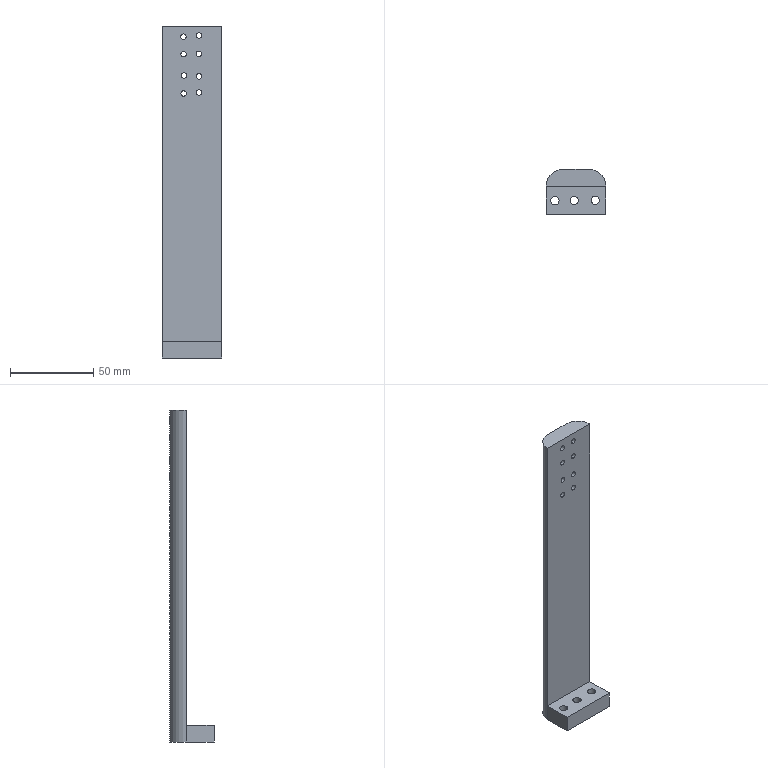Part | STEP file | L3.STEP | 1 solid | 32 faces | box 36 x 26.813 x 200 mm | volume 68195 mm3 | cylinder 24 | plane 8 | commonest cylinder face diameters 3.3 x16 5 x6 20 x2
STEP:
#1=CARTESIAN_POINT('',(-5.181,5.,191.886));
#2=VERTEX_POINT('',#1);
#3=CARTESIAN_POINT('',(-5.181,15.,191.886));
#4=VERTEX_POINT('',#3);
#5=CARTESIAN_POINT('',(-5.181,15.,191.886));
#6=DIRECTION('',(0.,1.,0.));
#7=VECTOR('',#6,1000.);
#8=LINE('',#5,#7);
#9=EDGE_CURVE('',#2,#4,#8,.T.);
#10=ORIENTED_EDGE('',*,*,#9,.F.);
#11=CARTESIAN_POINT('',(-5.181,5.,195.186));
#12=VERTEX_POINT('',#11);
#13=CARTESIAN_POINT('',(-5.181,5.,193.536));
#14=DIRECTION('',(0.,1.,0.));
#15=DIRECTION('',(0.,0.,1.));
#16=AXIS2_PLACEMENT_3D('',#13,#14,#15);
#17=CIRCLE('',#16,1.65);
#18=EDGE_CURVE('',#12,#2,#17,.T.);
#19=ORIENTED_EDGE('',*,*,#18,.F.);
#20=CARTESIAN_POINT('',(-5.181,15.,195.186));
#21=VERTEX_POINT('',#20);
#22=CARTESIAN_POINT('',(-5.181,15.,195.186));
#23=DIRECTION('',(0.,1.,0.));
#24=VECTOR('',#23,1000.);
#25=LINE('',#22,#24);
#26=EDGE_CURVE('',#12,#21,#25,.T.);
#27=ORIENTED_EDGE('',*,*,#26,.T.);
#28=CARTESIAN_POINT('',(-5.181,15.,193.536));
#29=DIRECTION('',(0.,1.,0.));
#30=DIRECTION('',(0.,0.,1.));
#31=AXIS2_PLACEMENT_3D('',#28,#29,#30);
#32=CIRCLE('',#31,1.65);
#33=EDGE_CURVE('',#21,#4,#32,.T.);
#34=ORIENTED_EDGE('',*,*,#33,.T.);
#35=EDGE_LOOP('',(#10,#19,#27,#34));
#36=FACE_OUTER_BOUND('',#35,.T.);
#37=CARTESIAN_POINT('',(-5.181,15.,193.536));
#38=DIRECTION('',(0.,1.,0.));
#39=DIRECTION('',(0.,0.,1.));
#40=AXIS2_PLACEMENT_3D('',#37,#38,#39);
#41=CYLINDRICAL_SURFACE('',#40,1.65);
#42=ADVANCED_FACE('',(#36),#41,.F.);
#43=CARTESIAN_POINT('',(4.086,5.,192.622));
#44=VERTEX_POINT('',#43);
#45=CARTESIAN_POINT('',(4.086,15.,192.622));
#46=VERTEX_POINT('',#45);
#47=CARTESIAN_POINT('',(4.086,15.,192.622));
#48=DIRECTION('',(0.,1.,0.));
#49=VECTOR('',#48,1000.);
#50=LINE('',#47,#49);
#51=EDGE_CURVE('',#44,#46,#50,.T.);
#52=ORIENTED_EDGE('',*,*,#51,.F.);
#53=CARTESIAN_POINT('',(4.086,5.,195.922));
#54=VERTEX_POINT('',#53);
#55=CARTESIAN_POINT('',(4.086,5.,194.272));
#56=DIRECTION('',(0.,1.,0.));
#57=DIRECTION('',(0.,0.,1.));
#58=AXIS2_PLACEMENT_3D('',#55,#56,#57);
#59=CIRCLE('',#58,1.65);
#60=EDGE_CURVE('',#54,#44,#59,.T.);
#61=ORIENTED_EDGE('',*,*,#60,.F.);
#62=CARTESIAN_POINT('',(4.086,15.,195.922));
#63=VERTEX_POINT('',#62);
#64=CARTESIAN_POINT('',(4.086,15.,195.922));
#65=DIRECTION('',(0.,1.,0.));
#66=VECTOR('',#65,1000.);
#67=LINE('',#64,#66);
#68=EDGE_CURVE('',#54,#63,#67,.T.);
#69=ORIENTED_EDGE('',*,*,#68,.T.);
#70=CARTESIAN_POINT('',(4.086,15.,194.272));
#71=DIRECTION('',(0.,1.,0.));
#72=DIRECTION('',(0.,0.,1.));
#73=AXIS2_PLACEMENT_3D('',#70,#71,#72);
#74=CIRCLE('',#73,1.65);
#75=EDGE_CURVE('',#63,#46,#74,.T.);
#76=ORIENTED_EDGE('',*,*,#75,.T.);
#77=EDGE_LOOP('',(#52,#61,#69,#76));
#78=FACE_OUTER_BOUND('',#77,.T.);
#79=CARTESIAN_POINT('',(4.086,15.,194.272));
#80=DIRECTION('',(0.,1.,0.));
#81=DIRECTION('',(0.,0.,1.));
#82=AXIS2_PLACEMENT_3D('',#79,#80,#81);
#83=CYLINDRICAL_SURFACE('',#82,1.65);
#84=ADVANCED_FACE('',(#78),#83,.F.);
#85=CARTESIAN_POINT('',(-5.004,5.,181.372));
#86=VERTEX_POINT('',#85);
#87=CARTESIAN_POINT('',(-5.004,15.,181.372));
#88=VERTEX_POINT('',#87);
#89=CARTESIAN_POINT('',(-5.004,15.,181.372));
#90=DIRECTION('',(0.,1.,0.));
#91=VECTOR('',#90,1000.);
#92=LINE('',#89,#91);
#93=EDGE_CURVE('',#86,#88,#92,.T.);
#94=ORIENTED_EDGE('',*,*,#93,.F.);
#95=CARTESIAN_POINT('',(-5.004,5.,184.672));
#96=VERTEX_POINT('',#95);
#97=CARTESIAN_POINT('',(-5.004,5.,183.022));
#98=DIRECTION('',(0.,1.,0.));
#99=DIRECTION('',(0.,0.,1.));
#100=AXIS2_PLACEMENT_3D('',#97,#98,#99);
#101=CIRCLE('',#100,1.65);
#102=EDGE_CURVE('',#96,#86,#101,.T.);
#103=ORIENTED_EDGE('',*,*,#102,.F.);
#104=CARTESIAN_POINT('',(-5.004,15.,184.672));
#105=VERTEX_POINT('',#104);
#106=CARTESIAN_POINT('',(-5.004,15.,184.672));
#107=DIRECTION('',(0.,1.,0.));
#108=VECTOR('',#107,1000.);
#109=LINE('',#106,#108);
#110=EDGE_CURVE('',#96,#105,#109,.T.);
#111=ORIENTED_EDGE('',*,*,#110,.T.);
#112=CARTESIAN_POINT('',(-5.004,15.,183.022));
#113=DIRECTION('',(0.,1.,0.));
#114=DIRECTION('',(0.,0.,1.));
#115=AXIS2_PLACEMENT_3D('',#112,#113,#114);
#116=CIRCLE('',#115,1.65);
#117=EDGE_CURVE('',#105,#88,#116,.T.);
#118=ORIENTED_EDGE('',*,*,#117,.T.);
#119=EDGE_LOOP('',(#94,#103,#111,#118));
#120=FACE_OUTER_BOUND('',#119,.T.);
#121=CARTESIAN_POINT('',(-5.004,15.,183.022));
#122=DIRECTION('',(0.,1.,0.));
#123=DIRECTION('',(0.,0.,1.));
#124=AXIS2_PLACEMENT_3D('',#121,#122,#123);
#125=CYLINDRICAL_SURFACE('',#124,1.65);
#126=ADVANCED_FACE('',(#120),#125,.F.);
#127=CARTESIAN_POINT('',(4.079,5.,181.598));
#128=VERTEX_POINT('',#127);
#129=CARTESIAN_POINT('',(4.079,15.,181.598));
#130=VERTEX_POINT('',#129);
#131=CARTESIAN_POINT('',(4.079,15.,181.598));
#132=DIRECTION('',(0.,1.,0.));
#133=VECTOR('',#132,1000.);
#134=LINE('',#131,#133);
#135=EDGE_CURVE('',#128,#130,#134,.T.);
#136=ORIENTED_EDGE('',*,*,#135,.F.);
#137=CARTESIAN_POINT('',(4.079,5.,184.898));
#138=VERTEX_POINT('',#137);
#139=CARTESIAN_POINT('',(4.079,5.,183.248));
#140=DIRECTION('',(0.,1.,0.));
#141=DIRECTION('',(0.,0.,1.));
#142=AXIS2_PLACEMENT_3D('',#139,#140,#141);
#143=CIRCLE('',#142,1.65);
#144=EDGE_CURVE('',#138,#128,#143,.T.);
#145=ORIENTED_EDGE('',*,*,#144,.F.);
#146=CARTESIAN_POINT('',(4.079,15.,184.898));
#147=VERTEX_POINT('',#146);
#148=CARTESIAN_POINT('',(4.079,15.,184.898));
#149=DIRECTION('',(0.,1.,0.));
#150=VECTOR('',#149,1000.);
#151=LINE('',#148,#150);
#152=EDGE_CURVE('',#138,#147,#151,.T.);
#153=ORIENTED_EDGE('',*,*,#152,.T.);
#154=CARTESIAN_POINT('',(4.079,15.,183.248));
#155=DIRECTION('',(0.,1.,0.));
#156=DIRECTION('',(0.,0.,1.));
#157=AXIS2_PLACEMENT_3D('',#154,#155,#156);
#158=CIRCLE('',#157,1.65);
#159=EDGE_CURVE('',#147,#130,#158,.T.);
#160=ORIENTED_EDGE('',*,*,#159,.T.);
#161=EDGE_LOOP('',(#136,#145,#153,#160));
#162=FACE_OUTER_BOUND('',#161,.T.);
#163=CARTESIAN_POINT('',(4.079,15.,183.248));
#164=DIRECTION('',(0.,1.,0.));
#165=DIRECTION('',(0.,0.,1.));
#166=AXIS2_PLACEMENT_3D('',#163,#164,#165);
#167=CYLINDRICAL_SURFACE('',#166,1.65);
#168=ADVANCED_FACE('',(#162),#167,.F.);
#169=CARTESIAN_POINT('',(4.196,5.,168.));
#170=VERTEX_POINT('',#169);
#171=CARTESIAN_POINT('',(4.196,15.,168.));
#172=VERTEX_POINT('',#171);
#173=CARTESIAN_POINT('',(4.196,15.,168.));
#174=DIRECTION('',(0.,1.,0.));
#175=VECTOR('',#174,1000.);
#176=LINE('',#173,#175);
#177=EDGE_CURVE('',#170,#172,#176,.T.);
#178=ORIENTED_EDGE('',*,*,#177,.F.);
#179=CARTESIAN_POINT('',(4.196,5.,171.3));
#180=VERTEX_POINT('',#179);
#181=CARTESIAN_POINT('',(4.196,5.,169.65));
#182=DIRECTION('',(0.,1.,0.));
#183=DIRECTION('',(0.,0.,1.));
#184=AXIS2_PLACEMENT_3D('',#181,#182,#183);
#185=CIRCLE('',#184,1.65);
#186=EDGE_CURVE('',#180,#170,#185,.T.);
#187=ORIENTED_EDGE('',*,*,#186,.F.);
#188=CARTESIAN_POINT('',(4.196,15.,171.3));
#189=VERTEX_POINT('',#188);
#190=CARTESIAN_POINT('',(4.196,15.,171.3));
#191=DIRECTION('',(0.,1.,0.));
#192=VECTOR('',#191,1000.);
#193=LINE('',#190,#192);
#194=EDGE_CURVE('',#180,#189,#193,.T.);
#195=ORIENTED_EDGE('',*,*,#194,.T.);
#196=CARTESIAN_POINT('',(4.196,15.,169.65));
#197=DIRECTION('',(0.,1.,0.));
#198=DIRECTION('',(0.,0.,1.));
#199=AXIS2_PLACEMENT_3D('',#196,#197,#198);
#200=CIRCLE('',#199,1.65);
#201=EDGE_CURVE('',#189,#172,#200,.T.);
#202=ORIENTED_EDGE('',*,*,#201,.T.);
#203=EDGE_LOOP('',(#178,#187,#195,#202));
#204=FACE_OUTER_BOUND('',#203,.T.);
#205=CARTESIAN_POINT('',(4.196,15.,169.65));
#206=DIRECTION('',(0.,1.,0.));
#207=DIRECTION('',(0.,0.,1.));
#208=AXIS2_PLACEMENT_3D('',#205,#206,#207);
#209=CYLINDRICAL_SURFACE('',#208,1.65);
#210=ADVANCED_FACE('',(#204),#209,.F.);
#211=CARTESIAN_POINT('',(-4.737,5.,168.514));
#212=VERTEX_POINT('',#211);
#213=CARTESIAN_POINT('',(-4.737,15.,168.514));
#214=VERTEX_POINT('',#213);
#215=CARTESIAN_POINT('',(-4.737,15.,168.514));
#216=DIRECTION('',(0.,1.,0.));
#217=VECTOR('',#216,1000.);
#218=LINE('',#215,#217);
#219=EDGE_CURVE('',#212,#214,#218,.T.);
#220=ORIENTED_EDGE('',*,*,#219,.F.);
#221=CARTESIAN_POINT('',(-4.737,5.,171.814));
#222=VERTEX_POINT('',#221);
#223=CARTESIAN_POINT('',(-4.737,5.,170.164));
#224=DIRECTION('',(0.,1.,0.));
#225=DIRECTION('',(0.,0.,1.));
#226=AXIS2_PLACEMENT_3D('',#223,#224,#225);
#227=CIRCLE('',#226,1.65);
#228=EDGE_CURVE('',#222,#212,#227,.T.);
#229=ORIENTED_EDGE('',*,*,#228,.F.);
#230=CARTESIAN_POINT('',(-4.737,15.,171.814));
#231=VERTEX_POINT('',#230);
#232=CARTESIAN_POINT('',(-4.737,15.,171.814));
#233=DIRECTION('',(0.,1.,0.));
#234=VECTOR('',#233,1000.);
#235=LINE('',#232,#234);
#236=EDGE_CURVE('',#222,#231,#235,.T.);
#237=ORIENTED_EDGE('',*,*,#236,.T.);
#238=CARTESIAN_POINT('',(-4.737,15.,170.164));
#239=DIRECTION('',(0.,1.,0.));
#240=DIRECTION('',(0.,0.,1.));
#241=AXIS2_PLACEMENT_3D('',#238,#239,#240);
#242=CIRCLE('',#241,1.65);
#243=EDGE_CURVE('',#231,#214,#242,.T.);
#244=ORIENTED_EDGE('',*,*,#243,.T.);
#245=EDGE_LOOP('',(#220,#229,#237,#244));
#246=FACE_OUTER_BOUND('',#245,.T.);
#247=CARTESIAN_POINT('',(-4.737,15.,170.164));
#248=DIRECTION('',(0.,1.,0.));
#249=DIRECTION('',(0.,0.,1.));
#250=AXIS2_PLACEMENT_3D('',#247,#248,#249);
#251=CYLINDRICAL_SURFACE('',#250,1.65);
#252=ADVANCED_FACE('',(#246),#251,.F.);
#253=CARTESIAN_POINT('',(4.08,5.,158.292));
#254=VERTEX_POINT('',#253);
#255=CARTESIAN_POINT('',(4.08,15.,158.292));
#256=VERTEX_POINT('',#255);
#257=CARTESIAN_POINT('',(4.08,15.,158.292));
#258=DIRECTION('',(0.,1.,0.));
#259=VECTOR('',#258,1000.);
#260=LINE('',#257,#259);
#261=EDGE_CURVE('',#254,#256,#260,.T.);
#262=ORIENTED_EDGE('',*,*,#261,.F.);
#263=CARTESIAN_POINT('',(4.08,5.,161.592));
#264=VERTEX_POINT('',#263);
#265=CARTESIAN_POINT('',(4.08,5.,159.942));
#266=DIRECTION('',(0.,1.,0.));
#267=DIRECTION('',(0.,0.,1.));
#268=AXIS2_PLACEMENT_3D('',#265,#266,#267);
#269=CIRCLE('',#268,1.65);
#270=EDGE_CURVE('',#264,#254,#269,.T.);
#271=ORIENTED_EDGE('',*,*,#270,.F.);
#272=CARTESIAN_POINT('',(4.08,15.,161.592));
#273=VERTEX_POINT('',#272);
#274=CARTESIAN_POINT('',(4.08,15.,161.592));
#275=DIRECTION('',(0.,1.,0.));
#276=VECTOR('',#275,1000.);
#277=LINE('',#274,#276);
#278=EDGE_CURVE('',#264,#273,#277,.T.);
#279=ORIENTED_EDGE('',*,*,#278,.T.);
#280=CARTESIAN_POINT('',(4.08,15.,159.942));
#281=DIRECTION('',(0.,1.,0.));
#282=DIRECTION('',(0.,0.,1.));
#283=AXIS2_PLACEMENT_3D('',#280,#281,#282);
#284=CIRCLE('',#283,1.65);
#285=EDGE_CURVE('',#273,#256,#284,.T.);
#286=ORIENTED_EDGE('',*,*,#285,.T.);
#287=EDGE_LOOP('',(#262,#271,#279,#286));
#288=FACE_OUTER_BOUND('',#287,.T.);
#289=CARTESIAN_POINT('',(4.08,15.,159.942));
#290=DIRECTION('',(0.,1.,0.));
#291=DIRECTION('',(0.,0.,1.));
#292=AXIS2_PLACEMENT_3D('',#289,#290,#291);
#293=CYLINDRICAL_SURFACE('',#292,1.65);
#294=ADVANCED_FACE('',(#288),#293,.F.);
#295=CARTESIAN_POINT('',(-5.03,5.,157.667));
#296=VERTEX_POINT('',#295);
#297=CARTESIAN_POINT('',(-5.03,15.,157.667));
#298=VERTEX_POINT('',#297);
#299=CARTESIAN_POINT('',(-5.03,15.,157.667));
#300=DIRECTION('',(0.,1.,0.));
#301=VECTOR('',#300,1000.);
#302=LINE('',#299,#301);
#303=EDGE_CURVE('',#296,#298,#302,.T.);
#304=ORIENTED_EDGE('',*,*,#303,.F.);
#305=CARTESIAN_POINT('',(-5.03,5.,160.967));
#306=VERTEX_POINT('',#305);
#307=CARTESIAN_POINT('',(-5.03,5.,159.317));
#308=DIRECTION('',(0.,1.,0.));
#309=DIRECTION('',(0.,0.,1.));
#310=AXIS2_PLACEMENT_3D('',#307,#308,#309);
#311=CIRCLE('',#310,1.65);
#312=EDGE_CURVE('',#306,#296,#311,.T.);
#313=ORIENTED_EDGE('',*,*,#312,.F.);
#314=CARTESIAN_POINT('',(-5.03,15.,160.967));
#315=VERTEX_POINT('',#314);
#316=CARTESIAN_POINT('',(-5.03,15.,160.967));
#317=DIRECTION('',(0.,1.,0.));
#318=VECTOR('',#317,1000.);
#319=LINE('',#316,#318);
#320=EDGE_CURVE('',#306,#315,#319,.T.);
#321=ORIENTED_EDGE('',*,*,#320,.T.);
#322=CARTESIAN_POINT('',(-5.03,15.,159.317));
#323=DIRECTION('',(0.,1.,0.));
#324=DIRECTION('',(0.,0.,1.));
#325=AXIS2_PLACEMENT_3D('',#322,#323,#324);
#326=CIRCLE('',#325,1.65);
#327=EDGE_CURVE('',#315,#298,#326,.T.);
#328=ORIENTED_EDGE('',*,*,#327,.T.);
#329=EDGE_LOOP('',(#304,#313,#321,#328));
#330=FACE_OUTER_BOUND('',#329,.T.);
#331=CARTESIAN_POINT('',(-5.03,15.,159.317));
#332=DIRECTION('',(0.,1.,0.));
#333=DIRECTION('',(0.,0.,1.));
#334=AXIS2_PLACEMENT_3D('',#331,#332,#333);
#335=CYLINDRICAL_SURFACE('',#334,1.65);
#336=ADVANCED_FACE('',(#330),#335,.F.);
#337=CARTESIAN_POINT('',(14.125,-3.204,10.));
#338=VERTEX_POINT('',#337);
#339=CARTESIAN_POINT('',(14.125,-3.204,0.));
#340=VERTEX_POINT('',#339);
#341=CARTESIAN_POINT('',(14.125,-3.204,0.));
#342=DIRECTION('',(0.,0.,-1.));
#343=VECTOR('',#342,1000.);
#344=LINE('',#341,#343);
#345=EDGE_CURVE('',#338,#340,#344,.T.);
#346=ORIENTED_EDGE('',*,*,#345,.F.);
#347=CARTESIAN_POINT('',(9.125,-3.204,10.));
#348=VERTEX_POINT('',#347);
#349=CARTESIAN_POINT('',(11.625,-3.204,10.));
#350=DIRECTION('',(0.,0.,-1.));
#351=DIRECTION('',(-1.,0.,0.));
#352=AXIS2_PLACEMENT_3D('',#349,#350,#351);
#353=CIRCLE('',#352,2.5);
#354=EDGE_CURVE('',#348,#338,#353,.T.);
#355=ORIENTED_EDGE('',*,*,#354,.F.);
#356=CARTESIAN_POINT('',(9.125,-3.204,0.));
#357=VERTEX_POINT('',#356);
#358=CARTESIAN_POINT('',(9.125,-3.204,0.));
#359=DIRECTION('',(0.,0.,-1.));
#360=VECTOR('',#359,1000.);
#361=LINE('',#358,#360);
#362=EDGE_CURVE('',#348,#357,#361,.T.);
#363=ORIENTED_EDGE('',*,*,#362,.T.);
#364=CARTESIAN_POINT('',(11.625,-3.204,0.));
#365=DIRECTION('',(0.,0.,-1.));
#366=DIRECTION('',(-1.,0.,0.));
#367=AXIS2_PLACEMENT_3D('',#364,#365,#366);
#368=CIRCLE('',#367,2.5);
#369=EDGE_CURVE('',#357,#340,#368,.T.);
#370=ORIENTED_EDGE('',*,*,#369,.T.);
#371=EDGE_LOOP('',(#346,#355,#363,#370));
#372=FACE_OUTER_BOUND('',#371,.T.);
#373=CARTESIAN_POINT('',(11.625,-3.204,0.));
#374=DIRECTION('',(0.,0.,-1.));
#375=DIRECTION('',(-1.,0.,0.));
#376=AXIS2_PLACEMENT_3D('',#373,#374,#375);
#377=CYLINDRICAL_SURFACE('',#376,2.5);
#378=ADVANCED_FACE('',(#372),#377,.F.);
#379=CARTESIAN_POINT('',(1.426,-3.367,10.));
#380=VERTEX_POINT('',#379);
#381=CARTESIAN_POINT('',(1.426,-3.367,0.));
#382=VERTEX_POINT('',#381);
#383=CARTESIAN_POINT('',(1.426,-3.367,0.));
#384=DIRECTION('',(0.,0.,-1.));
#385=VECTOR('',#384,1000.);
#386=LINE('',#383,#385);
#387=EDGE_CURVE('',#380,#382,#386,.T.);
#388=ORIENTED_EDGE('',*,*,#387,.F.);
#389=CARTESIAN_POINT('',(-3.574,-3.367,10.));
#390=VERTEX_POINT('',#389);
#391=CARTESIAN_POINT('',(-1.074,-3.367,10.));
#392=DIRECTION('',(0.,0.,-1.));
#393=DIRECTION('',(-1.,0.,0.));
#394=AXIS2_PLACEMENT_3D('',#391,#392,#393);
#395=CIRCLE('',#394,2.5);
#396=EDGE_CURVE('',#390,#380,#395,.T.);
#397=ORIENTED_EDGE('',*,*,#396,.F.);
#398=CARTESIAN_POINT('',(-3.574,-3.367,0.));
#399=VERTEX_POINT('',#398);
#400=CARTESIAN_POINT('',(-3.574,-3.367,0.));
#401=DIRECTION('',(0.,0.,-1.));
#402=VECTOR('',#401,1000.);
#403=LINE('',#400,#402);
#404=EDGE_CURVE('',#390,#399,#403,.T.);
#405=ORIENTED_EDGE('',*,*,#404,.T.);
#406=CARTESIAN_POINT('',(-1.074,-3.367,0.));
#407=DIRECTION('',(0.,0.,-1.));
#408=DIRECTION('',(-1.,0.,0.));
#409=AXIS2_PLACEMENT_3D('',#406,#407,#408);
#410=CIRCLE('',#409,2.5);
#411=EDGE_CURVE('',#399,#382,#410,.T.);
#412=ORIENTED_EDGE('',*,*,#411,.T.);
#413=EDGE_LOOP('',(#388,#397,#405,#412));
#414=FACE_OUTER_BOUND('',#413,.T.);
#415=CARTESIAN_POINT('',(-1.074,-3.367,0.));
#416=DIRECTION('',(0.,0.,-1.));
#417=DIRECTION('',(-1.,0.,0.));
#418=AXIS2_PLACEMENT_3D('',#415,#416,#417);
#419=CYLINDRICAL_SURFACE('',#418,2.5);
#420=ADVANCED_FACE('',(#414),#419,.F.);
#421=CARTESIAN_POINT('',(-10.172,-3.581,10.));
#422=VERTEX_POINT('',#421);
#423=CARTESIAN_POINT('',(-10.172,-3.581,0.));
#424=VERTEX_POINT('',#423);
#425=CARTESIAN_POINT('',(-10.172,-3.581,0.));
#426=DIRECTION('',(0.,0.,-1.));
#427=VECTOR('',#426,1000.);
#428=LINE('',#425,#427);
#429=EDGE_CURVE('',#422,#424,#428,.T.);
#430=ORIENTED_EDGE('',*,*,#429,.F.);
#431=CARTESIAN_POINT('',(-15.172,-3.581,10.));
#432=VERTEX_POINT('',#431);
#433=CARTESIAN_POINT('',(-12.672,-3.581,10.));
#434=DIRECTION('',(0.,0.,-1.));
#435=DIRECTION('',(-1.,0.,0.));
#436=AXIS2_PLACEMENT_3D('',#433,#434,#435);
#437=CIRCLE('',#436,2.5);
#438=EDGE_CURVE('',#432,#422,#437,.T.);
#439=ORIENTED_EDGE('',*,*,#438,.F.);
#440=CARTESIAN_POINT('',(-15.172,-3.581,0.));
#441=VERTEX_POINT('',#440);
#442=CARTESIAN_POINT('',(-15.172,-3.581,0.));
#443=DIRECTION('',(0.,0.,-1.));
#444=VECTOR('',#443,1000.);
#445=LINE('',#442,#444);
#446=EDGE_CURVE('',#432,#441,#445,.T.);
#447=ORIENTED_EDGE('',*,*,#446,.T.);
#448=CARTESIAN_POINT('',(-12.672,-3.581,0.));
#449=DIRECTION('',(0.,0.,-1.));
#450=DIRECTION('',(-1.,0.,0.));
#451=AXIS2_PLACEMENT_3D('',#448,#449,#450);
#452=CIRCLE('',#451,2.5);
#453=EDGE_CURVE('',#441,#424,#452,.T.);
#454=ORIENTED_EDGE('',*,*,#453,.T.);
#455=EDGE_LOOP('',(#430,#439,#447,#454));
#456=FACE_OUTER_BOUND('',#455,.T.);
#457=CARTESIAN_POINT('',(-12.672,-3.581,0.));
#458=DIRECTION('',(0.,0.,-1.));
#459=DIRECTION('',(-1.,0.,0.));
#460=AXIS2_PLACEMENT_3D('',#457,#458,#459);
#461=CYLINDRICAL_SURFACE('',#460,2.5);
#462=ADVANCED_FACE('',(#456),#461,.F.);
#463=ORIENTED_EDGE('',*,*,#438,.T.);
#464=CARTESIAN_POINT('',(-12.672,-3.581,10.));
#465=DIRECTION('',(0.,0.,-1.));
#466=DIRECTION('',(-1.,0.,0.));
#467=AXIS2_PLACEMENT_3D('',#464,#465,#466);
#468=CIRCLE('',#467,2.5);
#469=EDGE_CURVE('',#422,#432,#468,.T.);
#470=ORIENTED_EDGE('',*,*,#469,.T.);
#471=EDGE_LOOP('',(#463,#470));
#472=FACE_BOUND('',#471,.T.);
#473=ORIENTED_EDGE('',*,*,#396,.T.);
#474=CARTESIAN_POINT('',(-1.074,-3.367,10.));
#475=DIRECTION('',(0.,0.,-1.));
#476=DIRECTION('',(-1.,0.,0.));
#477=AXIS2_PLACEMENT_3D('',#474,#475,#476);
#478=CIRCLE('',#477,2.5);
#479=EDGE_CURVE('',#380,#390,#478,.T.);
#480=ORIENTED_EDGE('',*,*,#479,.T.);
#481=EDGE_LOOP('',(#473,#480));
#482=FACE_BOUND('',#481,.T.);
#483=ORIENTED_EDGE('',*,*,#354,.T.);
#484=CARTESIAN_POINT('',(11.625,-3.204,10.));
#485=DIRECTION('',(0.,0.,-1.));
#486=DIRECTION('',(-1.,0.,0.));
#487=AXIS2_PLACEMENT_3D('',#484,#485,#486);
#488=CIRCLE('',#487,2.5);
#489=EDGE_CURVE('',#338,#348,#488,.T.);
#490=ORIENTED_EDGE('',*,*,#489,.T.);
#491=EDGE_LOOP('',(#483,#490));
#492=FACE_BOUND('',#491,.T.);
#493=CARTESIAN_POINT('',(18.,5.,10.));
#494=VERTEX_POINT('',#493);
#495=CARTESIAN_POINT('',(18.,-11.813,10.));
#496=VERTEX_POINT('',#495);
#497=CARTESIAN_POINT('',(18.,5.,10.));
#498=DIRECTION('',(0.,-1.,0.));
#499=VECTOR('',#498,1000.);
#500=LINE('',#497,#499);
#501=EDGE_CURVE('',#494,#496,#500,.T.);
#502=ORIENTED_EDGE('',*,*,#501,.F.);
#503=CARTESIAN_POINT('',(-18.,5.,10.));
#504=VERTEX_POINT('',#503);
#505=CARTESIAN_POINT('',(18.,5.,10.));
#506=DIRECTION('',(1.,0.,0.));
#507=VECTOR('',#506,1000.);
#508=LINE('',#505,#507);
#509=EDGE_CURVE('',#504,#494,#508,.T.);
#510=ORIENTED_EDGE('',*,*,#509,.F.);
#511=CARTESIAN_POINT('',(-18.,-11.813,10.));
#512=VERTEX_POINT('',#511);
#513=CARTESIAN_POINT('',(-18.,5.,10.));
#514=DIRECTION('',(0.,1.,0.));
#515=VECTOR('',#514,1000.);
#516=LINE('',#513,#515);
#517=EDGE_CURVE('',#512,#504,#516,.T.);
#518=ORIENTED_EDGE('',*,*,#517,.F.);
#519=CARTESIAN_POINT('',(18.,-11.813,10.));
#520=DIRECTION('',(-1.,0.,0.));
#521=VECTOR('',#520,1000.);
#522=LINE('',#519,#521);
#523=EDGE_CURVE('',#496,#512,#522,.T.);
#524=ORIENTED_EDGE('',*,*,#523,.F.);
#525=EDGE_LOOP('',(#502,#510,#518,#524));
#526=FACE_OUTER_BOUND('',#525,.T.);
#527=CARTESIAN_POINT('',(0.,0.,10.));
#528=DIRECTION('',(0.,0.,-1.));
#529=DIRECTION('',(0.,-1.,0.));
#530=AXIS2_PLACEMENT_3D('',#527,#528,#529);
#531=PLANE('',#530);
#532=ADVANCED_FACE('',(#472,#482,#492,#526),#531,.F.);
#533=CARTESIAN_POINT('',(18.,-11.813,0.));
#534=VERTEX_POINT('',#533);
#535=CARTESIAN_POINT('',(-18.,-11.813,0.));
#536=VERTEX_POINT('',#535);
#537=CARTESIAN_POINT('',(18.,-11.813,0.));
#538=DIRECTION('',(-1.,0.,0.));
#539=VECTOR('',#538,1000.);
#540=LINE('',#537,#539);
#541=EDGE_CURVE('',#534,#536,#540,.T.);
#542=ORIENTED_EDGE('',*,*,#541,.F.);
#543=CARTESIAN_POINT('',(18.,-11.813,10.));
#544=DIRECTION('',(0.,0.,-1.));
#545=VECTOR('',#544,1000.);
#546=LINE('',#543,#545);
#547=EDGE_CURVE('',#496,#534,#546,.T.);
#548=ORIENTED_EDGE('',*,*,#547,.F.);
#549=ORIENTED_EDGE('',*,*,#523,.T.);
#550=CARTESIAN_POINT('',(-18.,-11.813,10.));
#551=DIRECTION('',(0.,0.,-1.));
#552=VECTOR('',#551,1000.);
#553=LINE('',#550,#552);
#554=EDGE_CURVE('',#512,#536,#553,.T.);
#555=ORIENTED_EDGE('',*,*,#554,.T.);
#556=EDGE_LOOP('',(#542,#548,#549,#555));
#557=FACE_OUTER_BOUND('',#556,.T.);
#558=CARTESIAN_POINT('',(18.,-11.813,10.));
#559=DIRECTION('',(0.,-1.,0.));
#560=DIRECTION('',(0.,0.,-1.));
#561=AXIS2_PLACEMENT_3D('',#558,#559,#560);
#562=PLANE('',#561);
#563=ADVANCED_FACE('',(#557),#562,.T.);
#564=CARTESIAN_POINT('',(-18.,5.,0.));
#565=VERTEX_POINT('',#564);
#566=CARTESIAN_POINT('',(-18.,5.,0.));
#567=DIRECTION('',(0.,1.,0.));
#568=VECTOR('',#567,1000.);
#569=LINE('',#566,#568);
#570=EDGE_CURVE('',#536,#565,#569,.T.);
#571=ORIENTED_EDGE('',*,*,#570,.F.);
#572=ORIENTED_EDGE('',*,*,#554,.F.);
#573=ORIENTED_EDGE('',*,*,#517,.T.);
#574=CARTESIAN_POINT('',(-18.,5.,10.));
#575=DIRECTION('',(0.,0.,-1.));
#576=VECTOR('',#575,1000.);
#577=LINE('',#574,#576);
#578=EDGE_CURVE('',#504,#565,#577,.T.);
#579=ORIENTED_EDGE('',*,*,#578,.T.);
#580=EDGE_LOOP('',(#571,#572,#573,#579));
#581=FACE_OUTER_BOUND('',#580,.T.);
#582=CARTESIAN_POINT('',(-18.,5.,10.));
#583=DIRECTION('',(-1.,0.,0.));
#584=DIRECTION('',(0.,0.,1.));
#585=AXIS2_PLACEMENT_3D('',#582,#583,#584);
#586=PLANE('',#585);
#587=ADVANCED_FACE('',(#581),#586,.T.);
#588=CARTESIAN_POINT('',(18.,5.,0.));
#589=VERTEX_POINT('',#588);
#590=CARTESIAN_POINT('',(18.,5.,0.));
#591=DIRECTION('',(0.,-1.,0.));
#592=VECTOR('',#591,1000.);
#593=LINE('',#590,#592);
#594=EDGE_CURVE('',#589,#534,#593,.T.);
#595=ORIENTED_EDGE('',*,*,#594,.F.);
#596=CARTESIAN_POINT('',(18.,5.,10.));
#597=DIRECTION('',(0.,0.,-1.));
#598=VECTOR('',#597,1000.);
#599=LINE('',#596,#598);
#600=EDGE_CURVE('',#494,#589,#599,.T.);
#601=ORIENTED_EDGE('',*,*,#600,.F.);
#602=ORIENTED_EDGE('',*,*,#501,.T.);
#603=ORIENTED_EDGE('',*,*,#547,.T.);
#604=EDGE_LOOP('',(#595,#601,#602,#603));
#605=FACE_OUTER_BOUND('',#604,.T.);
#606=CARTESIAN_POINT('',(18.,5.,10.));
#607=DIRECTION('',(1.,0.,0.));
#608=DIRECTION('',(0.,1.,0.));
#609=AXIS2_PLACEMENT_3D('',#606,#607,#608);
#610=PLANE('',#609);
#611=ADVANCED_FACE('',(#605),#610,.T.);
#612=ORIENTED_EDGE('',*,*,#453,.F.);
#613=CARTESIAN_POINT('',(-12.672,-3.581,0.));
#614=DIRECTION('',(0.,0.,-1.));
#615=DIRECTION('',(-1.,0.,0.));
#616=AXIS2_PLACEMENT_3D('',#613,#614,#615);
#617=CIRCLE('',#616,2.5);
#618=EDGE_CURVE('',#424,#441,#617,.T.);
#619=ORIENTED_EDGE('',*,*,#618,.F.);
#620=EDGE_LOOP('',(#612,#619));
#621=FACE_BOUND('',#620,.T.);
#622=ORIENTED_EDGE('',*,*,#411,.F.);
#623=CARTESIAN_POINT('',(-1.074,-3.367,0.));
#624=DIRECTION('',(0.,0.,-1.));
#625=DIRECTION('',(-1.,0.,0.));
#626=AXIS2_PLACEMENT_3D('',#623,#624,#625);
#627=CIRCLE('',#626,2.5);
#628=EDGE_CURVE('',#382,#399,#627,.T.);
#629=ORIENTED_EDGE('',*,*,#628,.F.);
#630=EDGE_LOOP('',(#622,#629));
#631=FACE_BOUND('',#630,.T.);
#632=ORIENTED_EDGE('',*,*,#369,.F.);
#633=CARTESIAN_POINT('',(11.625,-3.204,0.));
#634=DIRECTION('',(0.,0.,-1.));
#635=DIRECTION('',(-1.,0.,0.));
#636=AXIS2_PLACEMENT_3D('',#633,#634,#635);
#637=CIRCLE('',#636,2.5);
#638=EDGE_CURVE('',#340,#357,#637,.T.);
#639=ORIENTED_EDGE('',*,*,#638,.F.);
#640=EDGE_LOOP('',(#632,#639));
#641=FACE_BOUND('',#640,.T.);
#642=CARTESIAN_POINT('',(-8.,15.,0.));
#643=VERTEX_POINT('',#642);
#644=CARTESIAN_POINT('',(8.,15.,0.));
#645=VERTEX_POINT('',#644);
#646=CARTESIAN_POINT('',(0.,15.,0.));
#647=DIRECTION('',(1.,0.,0.));
#648=VECTOR('',#647,1000.);
#649=LINE('',#646,#648);
#650=EDGE_CURVE('',#643,#645,#649,.T.);
#651=ORIENTED_EDGE('',*,*,#650,.T.);
#652=CARTESIAN_POINT('',(8.,5.,0.));
#653=DIRECTION('',(0.,0.,-1.));
#654=DIRECTION('',(1.,0.,0.));
#655=AXIS2_PLACEMENT_3D('',#652,#653,#654);
#656=CIRCLE('',#655,10.);
#657=EDGE_CURVE('',#645,#589,#656,.T.);
#658=ORIENTED_EDGE('',*,*,#657,.T.);
#659=ORIENTED_EDGE('',*,*,#594,.T.);
#660=ORIENTED_EDGE('',*,*,#541,.T.);
#661=ORIENTED_EDGE('',*,*,#570,.T.);
#662=CARTESIAN_POINT('',(-8.,5.,0.));
#663=DIRECTION('',(0.,0.,1.));
#664=DIRECTION('',(1.,0.,0.));
#665=AXIS2_PLACEMENT_3D('',#662,#663,#664);
#666=CIRCLE('',#665,10.);
#667=EDGE_CURVE('',#643,#565,#666,.T.);
#668=ORIENTED_EDGE('',*,*,#667,.F.);
#669=EDGE_LOOP('',(#651,#658,#659,#660,#661,#668));
#670=FACE_OUTER_BOUND('',#669,.T.);
#671=CARTESIAN_POINT('',(0.,0.,0.));
#672=DIRECTION('',(0.,0.,1.));
#673=DIRECTION('',(1.,0.,0.));
#674=AXIS2_PLACEMENT_3D('',#671,#672,#673);
#675=PLANE('',#674);
#676=ADVANCED_FACE('',(#621,#631,#641,#670),#675,.F.);
#677=CARTESIAN_POINT('',(-8.,15.,200.));
#678=VERTEX_POINT('',#677);
#679=CARTESIAN_POINT('',(8.,15.,200.));
#680=VERTEX_POINT('',#679);
#681=CARTESIAN_POINT('',(0.,15.,200.));
#682=DIRECTION('',(1.,0.,0.));
#683=VECTOR('',#682,1000.);
#684=LINE('',#681,#683);
#685=EDGE_CURVE('',#678,#680,#684,.T.);
#686=ORIENTED_EDGE('',*,*,#685,.F.);
#687=CARTESIAN_POINT('',(-18.,5.,200.));
#688=VERTEX_POINT('',#687);
#689=CARTESIAN_POINT('',(-8.,5.,200.));
#690=DIRECTION('',(0.,0.,1.));
#691=DIRECTION('',(1.,0.,0.));
#692=AXIS2_PLACEMENT_3D('',#689,#690,#691);
#693=CIRCLE('',#692,10.);
#694=EDGE_CURVE('',#678,#688,#693,.T.);
#695=ORIENTED_EDGE('',*,*,#694,.T.);
#696=CARTESIAN_POINT('',(18.,5.,200.));
#697=VERTEX_POINT('',#696);
#698=CARTESIAN_POINT('',(0.,5.,200.));
#699=DIRECTION('',(1.,0.,0.));
#700=VECTOR('',#699,1000.);
#701=LINE('',#698,#700);
#702=EDGE_CURVE('',#688,#697,#701,.T.);
#703=ORIENTED_EDGE('',*,*,#702,.T.);
#704=CARTESIAN_POINT('',(8.,5.,200.));
#705=DIRECTION('',(0.,0.,-1.));
#706=DIRECTION('',(1.,0.,0.));
#707=AXIS2_PLACEMENT_3D('',#704,#705,#706);
#708=CIRCLE('',#707,10.);
#709=EDGE_CURVE('',#680,#697,#708,.T.);
#710=ORIENTED_EDGE('',*,*,#709,.F.);
#711=EDGE_LOOP('',(#686,#695,#703,#710));
#712=FACE_OUTER_BOUND('',#711,.T.);
#713=CARTESIAN_POINT('',(0.,0.,200.));
#714=DIRECTION('',(0.,0.,1.));
#715=DIRECTION('',(1.,0.,0.));
#716=AXIS2_PLACEMENT_3D('',#713,#714,#715);
#717=PLANE('',#716);
#718=ADVANCED_FACE('',(#712),#717,.T.);
#719=ORIENTED_EDGE('',*,*,#657,.F.);
#720=CARTESIAN_POINT('',(8.,15.,200.));
#721=DIRECTION('',(0.,0.,-1.));
#722=VECTOR('',#721,1000.);
#723=LINE('',#720,#722);
#724=EDGE_CURVE('',#680,#645,#723,.T.);
#725=ORIENTED_EDGE('',*,*,#724,.F.);
#726=ORIENTED_EDGE('',*,*,#709,.T.);
#727=CARTESIAN_POINT('',(18.,5.,200.));
#728=DIRECTION('',(0.,0.,-1.));
#729=VECTOR('',#728,1000.);
#730=LINE('',#727,#729);
#731=EDGE_CURVE('',#697,#494,#730,.T.);
#732=ORIENTED_EDGE('',*,*,#731,.T.);
#733=ORIENTED_EDGE('',*,*,#600,.T.);
#734=EDGE_LOOP('',(#719,#725,#726,#732,#733));
#735=FACE_OUTER_BOUND('',#734,.T.);
#736=CARTESIAN_POINT('',(8.,5.,200.));
#737=DIRECTION('',(0.,0.,-1.));
#738=DIRECTION('',(-1.,0.,0.));
#739=AXIS2_PLACEMENT_3D('',#736,#737,#738);
#740=CYLINDRICAL_SURFACE('',#739,10.);
#741=ADVANCED_FACE('',(#735),#740,.T.);
#742=ORIENTED_EDGE('',*,*,#312,.T.);
#743=CARTESIAN_POINT('',(-5.03,5.,159.317));
#744=DIRECTION('',(0.,1.,0.));
#745=DIRECTION('',(0.,0.,1.));
#746=AXIS2_PLACEMENT_3D('',#743,#744,#745);
#747=CIRCLE('',#746,1.65);
#748=EDGE_CURVE('',#296,#306,#747,.T.);
#749=ORIENTED_EDGE('',*,*,#748,.T.);
#750=EDGE_LOOP('',(#742,#749));
#751=FACE_BOUND('',#750,.T.);
#752=ORIENTED_EDGE('',*,*,#270,.T.);
#753=CARTESIAN_POINT('',(4.08,5.,159.942));
#754=DIRECTION('',(0.,1.,0.));
#755=DIRECTION('',(0.,0.,1.));
#756=AXIS2_PLACEMENT_3D('',#753,#754,#755);
#757=CIRCLE('',#756,1.65);
#758=EDGE_CURVE('',#254,#264,#757,.T.);
#759=ORIENTED_EDGE('',*,*,#758,.T.);
#760=EDGE_LOOP('',(#752,#759));
#761=FACE_BOUND('',#760,.T.);
#762=ORIENTED_EDGE('',*,*,#228,.T.);
#763=CARTESIAN_POINT('',(-4.737,5.,170.164));
#764=DIRECTION('',(0.,1.,0.));
#765=DIRECTION('',(0.,0.,1.));
#766=AXIS2_PLACEMENT_3D('',#763,#764,#765);
#767=CIRCLE('',#766,1.65);
#768=EDGE_CURVE('',#212,#222,#767,.T.);
#769=ORIENTED_EDGE('',*,*,#768,.T.);
#770=EDGE_LOOP('',(#762,#769));
#771=FACE_BOUND('',#770,.T.);
#772=ORIENTED_EDGE('',*,*,#186,.T.);
#773=CARTESIAN_POINT('',(4.196,5.,169.65));
#774=DIRECTION('',(0.,1.,0.));
#775=DIRECTION('',(0.,0.,1.));
#776=AXIS2_PLACEMENT_3D('',#773,#774,#775);
#777=CIRCLE('',#776,1.65);
#778=EDGE_CURVE('',#170,#180,#777,.T.);
#779=ORIENTED_EDGE('',*,*,#778,.T.);
#780=EDGE_LOOP('',(#772,#779));
#781=FACE_BOUND('',#780,.T.);
#782=ORIENTED_EDGE('',*,*,#144,.T.);
#783=CARTESIAN_POINT('',(4.079,5.,183.248));
#784=DIRECTION('',(0.,1.,0.));
#785=DIRECTION('',(0.,0.,1.));
#786=AXIS2_PLACEMENT_3D('',#783,#784,#785);
#787=CIRCLE('',#786,1.65);
#788=EDGE_CURVE('',#128,#138,#787,.T.);
#789=ORIENTED_EDGE('',*,*,#788,.T.);
#790=EDGE_LOOP('',(#782,#789));
#791=FACE_BOUND('',#790,.T.);
#792=ORIENTED_EDGE('',*,*,#102,.T.);
#793=CARTESIAN_POINT('',(-5.004,5.,183.022));
#794=DIRECTION('',(0.,1.,0.));
#795=DIRECTION('',(0.,0.,1.));
#796=AXIS2_PLACEMENT_3D('',#793,#794,#795);
#797=CIRCLE('',#796,1.65);
#798=EDGE_CURVE('',#86,#96,#797,.T.);
#799=ORIENTED_EDGE('',*,*,#798,.T.);
#800=EDGE_LOOP('',(#792,#799));
#801=FACE_BOUND('',#800,.T.);
#802=ORIENTED_EDGE('',*,*,#60,.T.);
#803=CARTESIAN_POINT('',(4.086,5.,194.272));
#804=DIRECTION('',(0.,1.,0.));
#805=DIRECTION('',(0.,0.,1.));
#806=AXIS2_PLACEMENT_3D('',#803,#804,#805);
#807=CIRCLE('',#806,1.65);
#808=EDGE_CURVE('',#44,#54,#807,.T.);
#809=ORIENTED_EDGE('',*,*,#808,.T.);
#810=EDGE_LOOP('',(#802,#809));
#811=FACE_BOUND('',#810,.T.);
#812=ORIENTED_EDGE('',*,*,#18,.T.);
#813=CARTESIAN_POINT('',(-5.181,5.,193.536));
#814=DIRECTION('',(0.,1.,0.));
#815=DIRECTION('',(0.,0.,1.));
#816=AXIS2_PLACEMENT_3D('',#813,#814,#815);
#817=CIRCLE('',#816,1.65);
#818=EDGE_CURVE('',#2,#12,#817,.T.);
#819=ORIENTED_EDGE('',*,*,#818,.T.);
#820=EDGE_LOOP('',(#812,#819));
#821=FACE_BOUND('',#820,.T.);
#822=CARTESIAN_POINT('',(-18.,5.,200.));
#823=DIRECTION('',(0.,0.,-1.));
#824=VECTOR('',#823,1000.);
#825=LINE('',#822,#824);
#826=EDGE_CURVE('',#688,#504,#825,.T.);
#827=ORIENTED_EDGE('',*,*,#826,.T.);
#828=ORIENTED_EDGE('',*,*,#509,.T.);
#829=ORIENTED_EDGE('',*,*,#731,.F.);
#830=ORIENTED_EDGE('',*,*,#702,.F.);
#831=EDGE_LOOP('',(#827,#828,#829,#830));
#832=FACE_OUTER_BOUND('',#831,.T.);
#833=CARTESIAN_POINT('',(0.,5.,200.));
#834=DIRECTION('',(0.,1.,0.));
#835=DIRECTION('',(1.,0.,0.));
#836=AXIS2_PLACEMENT_3D('',#833,#834,#835);
#837=PLANE('',#836);
#838=ADVANCED_FACE('',(#751,#761,#771,#781,#791,#801,#811,#821,#832),#837,.F.);
#839=ORIENTED_EDGE('',*,*,#667,.T.);
#840=ORIENTED_EDGE('',*,*,#578,.F.);
#841=ORIENTED_EDGE('',*,*,#826,.F.);
#842=ORIENTED_EDGE('',*,*,#694,.F.);
#843=CARTESIAN_POINT('',(-8.,15.,200.));
#844=DIRECTION('',(0.,0.,-1.));
#845=VECTOR('',#844,1000.);
#846=LINE('',#843,#845);
#847=EDGE_CURVE('',#678,#643,#846,.T.);
#848=ORIENTED_EDGE('',*,*,#847,.T.);
#849=EDGE_LOOP('',(#839,#840,#841,#842,#848));
#850=FACE_OUTER_BOUND('',#849,.T.);
#851=CARTESIAN_POINT('',(-8.,5.,200.));
#852=DIRECTION('',(0.,0.,-1.));
#853=DIRECTION('',(-1.,0.,0.));
#854=AXIS2_PLACEMENT_3D('',#851,#852,#853);
#855=CYLINDRICAL_SURFACE('',#854,10.);
#856=ADVANCED_FACE('',(#850),#855,.T.);
#857=ORIENTED_EDGE('',*,*,#327,.F.);
#858=CARTESIAN_POINT('',(-5.03,15.,159.317));
#859=DIRECTION('',(0.,1.,0.));
#860=DIRECTION('',(0.,0.,1.));
#861=AXIS2_PLACEMENT_3D('',#858,#859,#860);
#862=CIRCLE('',#861,1.65);
#863=EDGE_CURVE('',#298,#315,#862,.T.);
#864=ORIENTED_EDGE('',*,*,#863,.F.);
#865=EDGE_LOOP('',(#857,#864));
#866=FACE_BOUND('',#865,.T.);
#867=ORIENTED_EDGE('',*,*,#285,.F.);
#868=CARTESIAN_POINT('',(4.08,15.,159.942));
#869=DIRECTION('',(0.,1.,0.));
#870=DIRECTION('',(0.,0.,1.));
#871=AXIS2_PLACEMENT_3D('',#868,#869,#870);
#872=CIRCLE('',#871,1.65);
#873=EDGE_CURVE('',#256,#273,#872,.T.);
#874=ORIENTED_EDGE('',*,*,#873,.F.);
#875=EDGE_LOOP('',(#867,#874));
#876=FACE_BOUND('',#875,.T.);
#877=ORIENTED_EDGE('',*,*,#243,.F.);
#878=CARTESIAN_POINT('',(-4.737,15.,170.164));
#879=DIRECTION('',(0.,1.,0.));
#880=DIRECTION('',(0.,0.,1.));
#881=AXIS2_PLACEMENT_3D('',#878,#879,#880);
#882=CIRCLE('',#881,1.65);
#883=EDGE_CURVE('',#214,#231,#882,.T.);
#884=ORIENTED_EDGE('',*,*,#883,.F.);
#885=EDGE_LOOP('',(#877,#884));
#886=FACE_BOUND('',#885,.T.);
#887=ORIENTED_EDGE('',*,*,#201,.F.);
#888=CARTESIAN_POINT('',(4.196,15.,169.65));
#889=DIRECTION('',(0.,1.,0.));
#890=DIRECTION('',(0.,0.,1.));
#891=AXIS2_PLACEMENT_3D('',#888,#889,#890);
#892=CIRCLE('',#891,1.65);
#893=EDGE_CURVE('',#172,#189,#892,.T.);
#894=ORIENTED_EDGE('',*,*,#893,.F.);
#895=EDGE_LOOP('',(#887,#894));
#896=FACE_BOUND('',#895,.T.);
#897=ORIENTED_EDGE('',*,*,#159,.F.);
#898=CARTESIAN_POINT('',(4.079,15.,183.248));
#899=DIRECTION('',(0.,1.,0.));
#900=DIRECTION('',(0.,0.,1.));
#901=AXIS2_PLACEMENT_3D('',#898,#899,#900);
#902=CIRCLE('',#901,1.65);
#903=EDGE_CURVE('',#130,#147,#902,.T.);
#904=ORIENTED_EDGE('',*,*,#903,.F.);
#905=EDGE_LOOP('',(#897,#904));
#906=FACE_BOUND('',#905,.T.);
#907=ORIENTED_EDGE('',*,*,#117,.F.);
#908=CARTESIAN_POINT('',(-5.004,15.,183.022));
#909=DIRECTION('',(0.,1.,0.));
#910=DIRECTION('',(0.,0.,1.));
#911=AXIS2_PLACEMENT_3D('',#908,#909,#910);
#912=CIRCLE('',#911,1.65);
#913=EDGE_CURVE('',#88,#105,#912,.T.);
#914=ORIENTED_EDGE('',*,*,#913,.F.);
#915=EDGE_LOOP('',(#907,#914));
#916=FACE_BOUND('',#915,.T.);
#917=ORIENTED_EDGE('',*,*,#75,.F.);
#918=CARTESIAN_POINT('',(4.086,15.,194.272));
#919=DIRECTION('',(0.,1.,0.));
#920=DIRECTION('',(0.,0.,1.));
#921=AXIS2_PLACEMENT_3D('',#918,#919,#920);
#922=CIRCLE('',#921,1.65);
#923=EDGE_CURVE('',#46,#63,#922,.T.);
#924=ORIENTED_EDGE('',*,*,#923,.F.);
#925=EDGE_LOOP('',(#917,#924));
#926=FACE_BOUND('',#925,.T.);
#927=ORIENTED_EDGE('',*,*,#33,.F.);
#928=CARTESIAN_POINT('',(-5.181,15.,193.536));
#929=DIRECTION('',(0.,1.,0.));
#930=DIRECTION('',(0.,0.,1.));
#931=AXIS2_PLACEMENT_3D('',#928,#929,#930);
#932=CIRCLE('',#931,1.65);
#933=EDGE_CURVE('',#4,#21,#932,.T.);
#934=ORIENTED_EDGE('',*,*,#933,.F.);
#935=EDGE_LOOP('',(#927,#934));
#936=FACE_BOUND('',#935,.T.);
#937=ORIENTED_EDGE('',*,*,#650,.F.);
#938=ORIENTED_EDGE('',*,*,#847,.F.);
#939=ORIENTED_EDGE('',*,*,#685,.T.);
#940=ORIENTED_EDGE('',*,*,#724,.T.);
#941=EDGE_LOOP('',(#937,#938,#939,#940));
#942=FACE_OUTER_BOUND('',#941,.T.);
#943=CARTESIAN_POINT('',(0.,15.,200.));
#944=DIRECTION('',(0.,1.,0.));
#945=DIRECTION('',(1.,0.,0.));
#946=AXIS2_PLACEMENT_3D('',#943,#944,#945);
#947=PLANE('',#946);
#948=ADVANCED_FACE('',(#866,#876,#886,#896,#906,#916,#926,#936,#942),#947,.T.);
#949=ORIENTED_EDGE('',*,*,#469,.F.);
#950=ORIENTED_EDGE('',*,*,#429,.T.);
#951=ORIENTED_EDGE('',*,*,#618,.T.);
#952=ORIENTED_EDGE('',*,*,#446,.F.);
#953=EDGE_LOOP('',(#949,#950,#951,#952));
#954=FACE_OUTER_BOUND('',#953,.T.);
#955=CARTESIAN_POINT('',(-12.672,-3.581,0.));
#956=DIRECTION('',(0.,0.,-1.));
#957=DIRECTION('',(-1.,0.,0.));
#958=AXIS2_PLACEMENT_3D('',#955,#956,#957);
#959=CYLINDRICAL_SURFACE('',#958,2.5);
#960=ADVANCED_FACE('',(#954),#959,.F.);
#961=ORIENTED_EDGE('',*,*,#479,.F.);
#962=ORIENTED_EDGE('',*,*,#387,.T.);
#963=ORIENTED_EDGE('',*,*,#628,.T.);
#964=ORIENTED_EDGE('',*,*,#404,.F.);
#965=EDGE_LOOP('',(#961,#962,#963,#964));
#966=FACE_OUTER_BOUND('',#965,.T.);
#967=CARTESIAN_POINT('',(-1.074,-3.367,0.));
#968=DIRECTION('',(0.,0.,-1.));
#969=DIRECTION('',(-1.,0.,0.));
#970=AXIS2_PLACEMENT_3D('',#967,#968,#969);
#971=CYLINDRICAL_SURFACE('',#970,2.5);
#972=ADVANCED_FACE('',(#966),#971,.F.);
#973=ORIENTED_EDGE('',*,*,#489,.F.);
#974=ORIENTED_EDGE('',*,*,#345,.T.);
#975=ORIENTED_EDGE('',*,*,#638,.T.);
#976=ORIENTED_EDGE('',*,*,#362,.F.);
#977=EDGE_LOOP('',(#973,#974,#975,#976));
#978=FACE_OUTER_BOUND('',#977,.T.);
#979=CARTESIAN_POINT('',(11.625,-3.204,0.));
#980=DIRECTION('',(0.,0.,-1.));
#981=DIRECTION('',(-1.,0.,0.));
#982=AXIS2_PLACEMENT_3D('',#979,#980,#981);
#983=CYLINDRICAL_SURFACE('',#982,2.5);
#984=ADVANCED_FACE('',(#978),#983,.F.);
#985=ORIENTED_EDGE('',*,*,#748,.F.);
#986=ORIENTED_EDGE('',*,*,#303,.T.);
#987=ORIENTED_EDGE('',*,*,#863,.T.);
#988=ORIENTED_EDGE('',*,*,#320,.F.);
#989=EDGE_LOOP('',(#985,#986,#987,#988));
#990=FACE_OUTER_BOUND('',#989,.T.);
#991=CARTESIAN_POINT('',(-5.03,15.,159.317));
#992=DIRECTION('',(0.,1.,0.));
#993=DIRECTION('',(0.,0.,1.));
#994=AXIS2_PLACEMENT_3D('',#991,#992,#993);
#995=CYLINDRICAL_SURFACE('',#994,1.65);
#996=ADVANCED_FACE('',(#990),#995,.F.);
#997=ORIENTED_EDGE('',*,*,#758,.F.);
#998=ORIENTED_EDGE('',*,*,#261,.T.);
#999=ORIENTED_EDGE('',*,*,#873,.T.);
#1000=ORIENTED_EDGE('',*,*,#278,.F.);
#1001=EDGE_LOOP('',(#997,#998,#999,#1000));
#1002=FACE_OUTER_BOUND('',#1001,.T.);
#1003=CARTESIAN_POINT('',(4.08,15.,159.942));
#1004=DIRECTION('',(0.,1.,0.));
#1005=DIRECTION('',(0.,0.,1.));
#1006=AXIS2_PLACEMENT_3D('',#1003,#1004,#1005);
#1007=CYLINDRICAL_SURFACE('',#1006,1.65);
#1008=ADVANCED_FACE('',(#1002),#1007,.F.);
#1009=ORIENTED_EDGE('',*,*,#768,.F.);
#1010=ORIENTED_EDGE('',*,*,#219,.T.);
#1011=ORIENTED_EDGE('',*,*,#883,.T.);
#1012=ORIENTED_EDGE('',*,*,#236,.F.);
#1013=EDGE_LOOP('',(#1009,#1010,#1011,#1012));
#1014=FACE_OUTER_BOUND('',#1013,.T.);
#1015=CARTESIAN_POINT('',(-4.737,15.,170.164));
#1016=DIRECTION('',(0.,1.,0.));
#1017=DIRECTION('',(0.,0.,1.));
#1018=AXIS2_PLACEMENT_3D('',#1015,#1016,#1017);
#1019=CYLINDRICAL_SURFACE('',#1018,1.65);
#1020=ADVANCED_FACE('',(#1014),#1019,.F.);
#1021=ORIENTED_EDGE('',*,*,#778,.F.);
#1022=ORIENTED_EDGE('',*,*,#177,.T.);
#1023=ORIENTED_EDGE('',*,*,#893,.T.);
#1024=ORIENTED_EDGE('',*,*,#194,.F.);
#1025=EDGE_LOOP('',(#1021,#1022,#1023,#1024));
#1026=FACE_OUTER_BOUND('',#1025,.T.);
#1027=CARTESIAN_POINT('',(4.196,15.,169.65));
#1028=DIRECTION('',(0.,1.,0.));
#1029=DIRECTION('',(0.,0.,1.));
#1030=AXIS2_PLACEMENT_3D('',#1027,#1028,#1029);
#1031=CYLINDRICAL_SURFACE('',#1030,1.65);
#1032=ADVANCED_FACE('',(#1026),#1031,.F.);
#1033=ORIENTED_EDGE('',*,*,#788,.F.);
#1034=ORIENTED_EDGE('',*,*,#135,.T.);
#1035=ORIENTED_EDGE('',*,*,#903,.T.);
#1036=ORIENTED_EDGE('',*,*,#152,.F.);
#1037=EDGE_LOOP('',(#1033,#1034,#1035,#1036));
#1038=FACE_OUTER_BOUND('',#1037,.T.);
#1039=CARTESIAN_POINT('',(4.079,15.,183.248));
#1040=DIRECTION('',(0.,1.,0.));
#1041=DIRECTION('',(0.,0.,1.));
#1042=AXIS2_PLACEMENT_3D('',#1039,#1040,#1041);
#1043=CYLINDRICAL_SURFACE('',#1042,1.65);
#1044=ADVANCED_FACE('',(#1038),#1043,.F.);
#1045=ORIENTED_EDGE('',*,*,#798,.F.);
#1046=ORIENTED_EDGE('',*,*,#93,.T.);
#1047=ORIENTED_EDGE('',*,*,#913,.T.);
#1048=ORIENTED_EDGE('',*,*,#110,.F.);
#1049=EDGE_LOOP('',(#1045,#1046,#1047,#1048));
#1050=FACE_OUTER_BOUND('',#1049,.T.);
#1051=CARTESIAN_POINT('',(-5.004,15.,183.022));
#1052=DIRECTION('',(0.,1.,0.));
#1053=DIRECTION('',(0.,0.,1.));
#1054=AXIS2_PLACEMENT_3D('',#1051,#1052,#1053);
#1055=CYLINDRICAL_SURFACE('',#1054,1.65);
#1056=ADVANCED_FACE('',(#1050),#1055,.F.);
#1057=ORIENTED_EDGE('',*,*,#808,.F.);
#1058=ORIENTED_EDGE('',*,*,#51,.T.);
#1059=ORIENTED_EDGE('',*,*,#923,.T.);
#1060=ORIENTED_EDGE('',*,*,#68,.F.);
#1061=EDGE_LOOP('',(#1057,#1058,#1059,#1060));
#1062=FACE_OUTER_BOUND('',#1061,.T.);
#1063=CARTESIAN_POINT('',(4.086,15.,194.272));
#1064=DIRECTION('',(0.,1.,0.));
#1065=DIRECTION('',(0.,0.,1.));
#1066=AXIS2_PLACEMENT_3D('',#1063,#1064,#1065);
#1067=CYLINDRICAL_SURFACE('',#1066,1.65);
#1068=ADVANCED_FACE('',(#1062),#1067,.F.);
#1069=ORIENTED_EDGE('',*,*,#818,.F.);
#1070=ORIENTED_EDGE('',*,*,#9,.T.);
#1071=ORIENTED_EDGE('',*,*,#933,.T.);
#1072=ORIENTED_EDGE('',*,*,#26,.F.);
#1073=EDGE_LOOP('',(#1069,#1070,#1071,#1072));
#1074=FACE_OUTER_BOUND('',#1073,.T.);
#1075=CARTESIAN_POINT('',(-5.181,15.,193.536));
#1076=DIRECTION('',(0.,1.,0.));
#1077=DIRECTION('',(0.,0.,1.));
#1078=AXIS2_PLACEMENT_3D('',#1075,#1076,#1077);
#1079=CYLINDRICAL_SURFACE('',#1078,1.65);
#1080=ADVANCED_FACE('',(#1074),#1079,.F.);
#1081=CLOSED_SHELL('',(#42,#84,#126,#168,#210,#252,#294,#336,#378,#420,#462,#532,#563,#587,#611,#676,#718,#741,#838,#856,#948,#960,#972,#984,#996,#1008,#1020,#1032,#1044,#1056,#1068,#1080));
#1082=MANIFOLD_SOLID_BREP('',#1081);
#1083=CARTESIAN_POINT('',(0.,0.,0.));
#1084=DIRECTION('',(0.,0.,1.));
#1085=DIRECTION('',(1.,0.,0.));
#1086=AXIS2_PLACEMENT_3D('',#1083,#1084,#1085);
#1087=(LENGTH_UNIT()NAMED_UNIT(*)SI_UNIT(.MILLI.,.METRE.));
#1088=UNCERTAINTY_MEASURE_WITH_UNIT(LENGTH_MEASURE(0.00001),#1087,'','');
#1089=(NAMED_UNIT(*)PLANE_ANGLE_UNIT()SI_UNIT($,.RADIAN.));
#1090=(NAMED_UNIT(*)SI_UNIT($,.STERADIAN.)SOLID_ANGLE_UNIT());
#1091=(GEOMETRIC_REPRESENTATION_CONTEXT(3)GLOBAL_UNCERTAINTY_ASSIGNED_CONTEXT((#1088))GLOBAL_UNIT_ASSIGNED_CONTEXT((#1087,#1089,#1090))REPRESENTATION_CONTEXT('',''));
#1092=ADVANCED_BREP_SHAPE_REPRESENTATION('',(#1082,#1086),#1091);